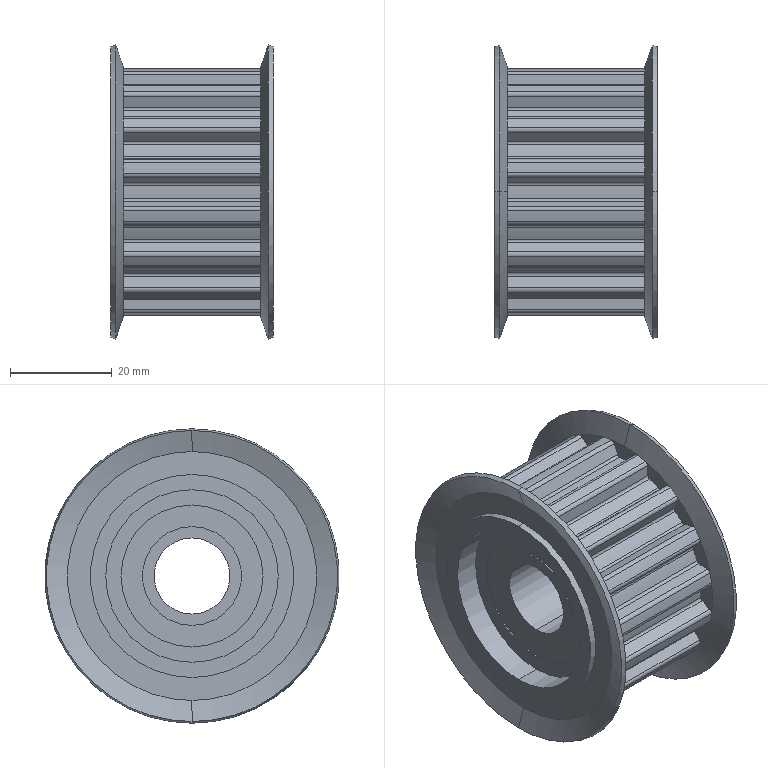Part | SolidWorks | features Revolution 4, ICE 2, CirPattern 1, RefAxis 1 | 2 solids | 209 faces | box 32 x 58 x 58 mm | volume 40036 mm3 | cylinder 120 | plane 77 | cone 12 | commonest cylinder face diameters 1.2 x32 1.6 x32 42.65 x16 49.05 x16 35 x6 19.5 x4